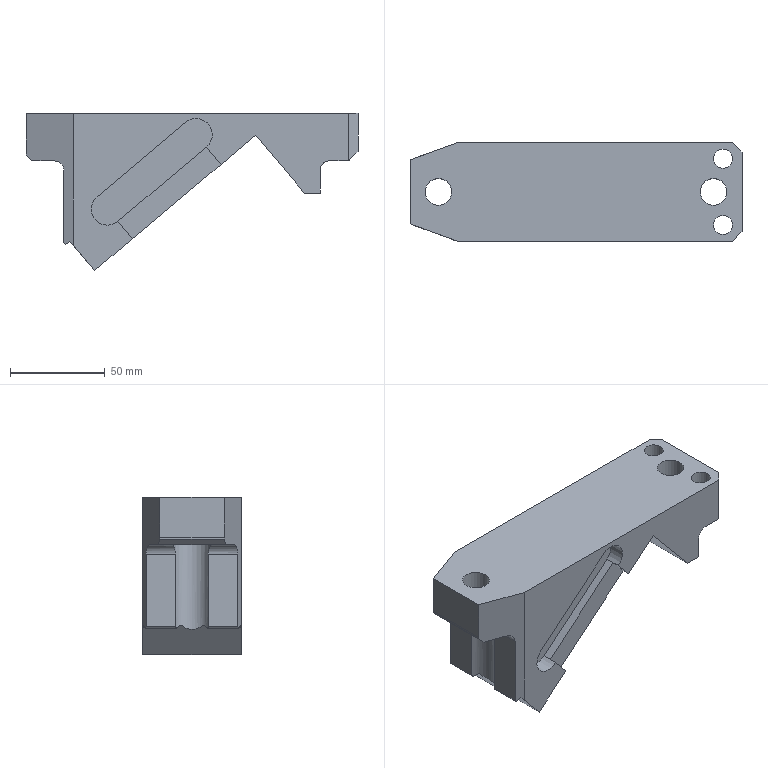Part | NX | features solid 2 | 1 solid | 61 faces | box 175 x 52 x 82.801 mm | volume 324369 mm3 | plane 45 | cylinder 16 | commonest cylinder face diameters 10 x6 17 x4 11 x2 14 x2 20 x2